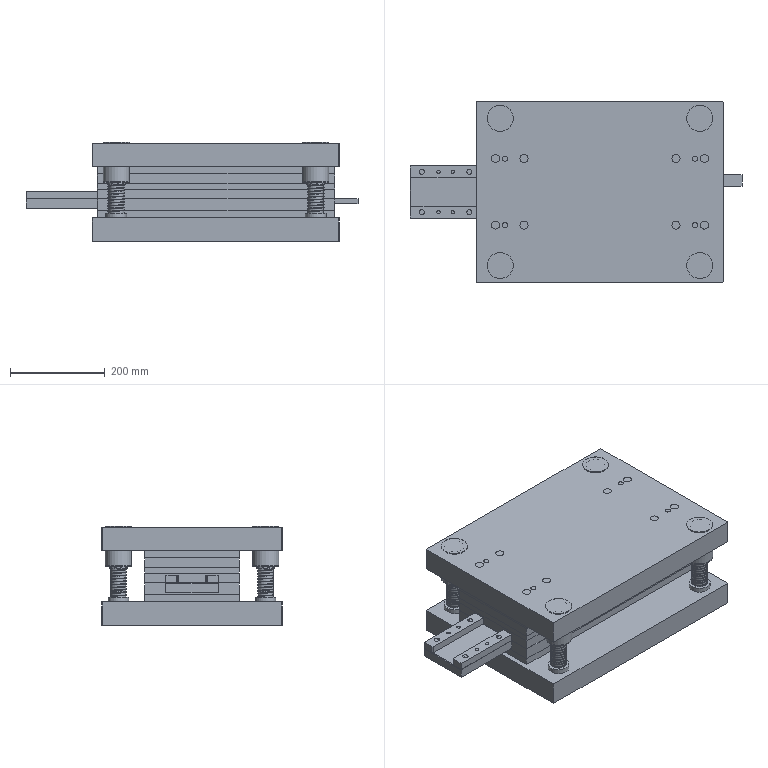Part | NX | features BREP 282 | 434 solids | 6821 faces | volume 34284775 mm3 | plane 3853 | cylinder 2136 | sphere 648 | cone 100 | torus 76 | spline 8 | commonest cylinder face diameters 1 x570 1.1 x224 0.9 x153 10 x88 3.1 x70 1.05 x65